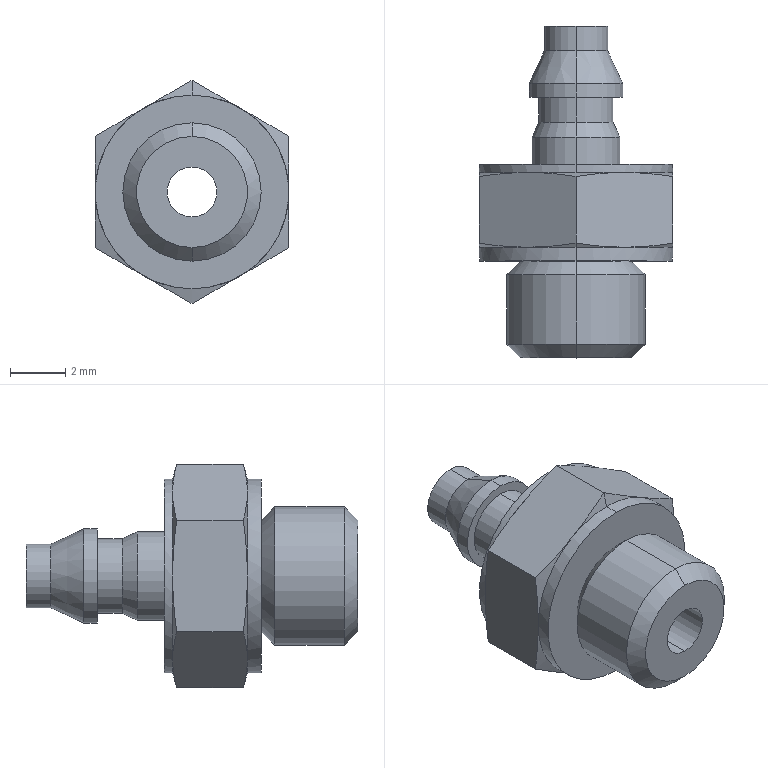Part | SolidWorks | features BaseBody 1 | 1 solid | 49 faces | box 7 x 12 x 8.083 mm | volume 212.301 mm3 | cone 22 | cylinder 16 | plane 11 | commonest cylinder face diameters 7 x4 1.8 x2 2.3 x2 2.7 x2 3.2 x2 3.4 x2
STEP:
#1=CARTESIAN_POINT('',(0.,-3.5,0.9));
#2=VERTEX_POINT('',#1);
#3=CARTESIAN_POINT('',(0.,-3.5,-0.9));
#4=VERTEX_POINT('',#3);
#5=CARTESIAN_POINT('',(0.,-3.5,0.));
#6=DIRECTION('',(0.,-1.,0.));
#7=DIRECTION('',(0.,0.,1.));
#8=AXIS2_PLACEMENT_3D('',#5,#6,#7);
#9=CIRCLE('',#8,0.9);
#10=EDGE_CURVE('',#2,#4,#9,.T.);
#11=ORIENTED_EDGE('',*,*,#10,.T.);
#12=CARTESIAN_POINT('',(0.,8.5,-0.9));
#13=VERTEX_POINT('',#12);
#14=CARTESIAN_POINT('',(0.,-3.5,-0.9));
#15=DIRECTION('',(0.,1.,0.));
#16=VECTOR('',#15,1000.);
#17=LINE('',#14,#16);
#18=EDGE_CURVE('',#4,#13,#17,.T.);
#19=ORIENTED_EDGE('',*,*,#18,.T.);
#20=CARTESIAN_POINT('',(0.,8.5,0.9));
#21=VERTEX_POINT('',#20);
#22=CARTESIAN_POINT('',(0.,8.5,0.));
#23=DIRECTION('',(0.,1.,0.));
#24=DIRECTION('',(0.,0.,1.));
#25=AXIS2_PLACEMENT_3D('',#22,#23,#24);
#26=CIRCLE('',#25,0.9);
#27=EDGE_CURVE('',#13,#21,#26,.T.);
#28=ORIENTED_EDGE('',*,*,#27,.T.);
#29=CARTESIAN_POINT('',(0.,-3.5,0.9));
#30=DIRECTION('',(0.,1.,0.));
#31=VECTOR('',#30,1000.);
#32=LINE('',#29,#31);
#33=EDGE_CURVE('',#2,#21,#32,.T.);
#34=ORIENTED_EDGE('',*,*,#33,.F.);
#35=EDGE_LOOP('',(#11,#19,#28,#34));
#36=FACE_OUTER_BOUND('',#35,.T.);
#37=CARTESIAN_POINT('',(0.,-3.5,0.));
#38=DIRECTION('',(0.,1.,0.));
#39=DIRECTION('',(0.,0.,1.));
#40=AXIS2_PLACEMENT_3D('',#37,#38,#39);
#41=CYLINDRICAL_SURFACE('',#40,0.9);
#42=ADVANCED_FACE('',(#36),#41,.F.);
#43=CARTESIAN_POINT('',(0.,7.6,1.15));
#44=VERTEX_POINT('',#43);
#45=CARTESIAN_POINT('',(0.,7.6,-1.15));
#46=VERTEX_POINT('',#45);
#47=CARTESIAN_POINT('',(0.,7.6,0.));
#48=DIRECTION('',(0.,1.,0.));
#49=DIRECTION('',(1.,0.,0.));
#50=AXIS2_PLACEMENT_3D('',#47,#48,#49);
#51=CIRCLE('',#50,1.15);
#52=EDGE_CURVE('',#44,#46,#51,.T.);
#53=ORIENTED_EDGE('',*,*,#52,.T.);
#54=CARTESIAN_POINT('',(0.,8.5,-1.15));
#55=VERTEX_POINT('',#54);
#56=CARTESIAN_POINT('',(0.,8.5,-1.15));
#57=DIRECTION('',(0.,1.,0.));
#58=VECTOR('',#57,1000.);
#59=LINE('',#56,#58);
#60=EDGE_CURVE('',#46,#55,#59,.T.);
#61=ORIENTED_EDGE('',*,*,#60,.T.);
#62=CARTESIAN_POINT('',(0.,8.5,1.15));
#63=VERTEX_POINT('',#62);
#64=CARTESIAN_POINT('',(0.,8.5,0.));
#65=DIRECTION('',(0.,1.,0.));
#66=DIRECTION('',(0.,0.,1.));
#67=AXIS2_PLACEMENT_3D('',#64,#65,#66);
#68=CIRCLE('',#67,1.15);
#69=EDGE_CURVE('',#63,#55,#68,.T.);
#70=ORIENTED_EDGE('',*,*,#69,.F.);
#71=CARTESIAN_POINT('',(0.,8.5,1.15));
#72=DIRECTION('',(0.,1.,0.));
#73=VECTOR('',#72,1000.);
#74=LINE('',#71,#73);
#75=EDGE_CURVE('',#44,#63,#74,.T.);
#76=ORIENTED_EDGE('',*,*,#75,.F.);
#77=EDGE_LOOP('',(#53,#61,#70,#76));
#78=FACE_OUTER_BOUND('',#77,.T.);
#79=CARTESIAN_POINT('',(0.,8.5,0.));
#80=DIRECTION('',(0.,1.,0.));
#81=DIRECTION('',(0.,0.,1.));
#82=AXIS2_PLACEMENT_3D('',#79,#80,#81);
#83=CYLINDRICAL_SURFACE('',#82,1.15);
#84=ADVANCED_FACE('',(#78),#83,.T.);
#85=CARTESIAN_POINT('',(0.,-3.5,-2.01));
#86=VERTEX_POINT('',#85);
#87=CARTESIAN_POINT('',(0.,-3.5,2.01));
#88=VERTEX_POINT('',#87);
#89=CARTESIAN_POINT('',(0.,-3.5,0.));
#90=DIRECTION('',(0.,-1.,0.));
#91=DIRECTION('',(0.,0.,1.));
#92=AXIS2_PLACEMENT_3D('',#89,#90,#91);
#93=CIRCLE('',#92,2.01);
#94=EDGE_CURVE('',#86,#88,#93,.T.);
#95=ORIENTED_EDGE('',*,*,#94,.F.);
#96=CARTESIAN_POINT('',(0.,-3.009,-2.5));
#97=VERTEX_POINT('',#96);
#98=CARTESIAN_POINT('',(0.,-3.5,-2.01));
#99=DIRECTION('',(0.,0.7071,-0.7071));
#100=VECTOR('',#99,1000.);
#101=LINE('',#98,#100);
#102=EDGE_CURVE('',#86,#97,#101,.T.);
#103=ORIENTED_EDGE('',*,*,#102,.T.);
#104=CARTESIAN_POINT('',(0.,-3.009,2.5));
#105=VERTEX_POINT('',#104);
#106=CARTESIAN_POINT('',(0.,-3.009,0.));
#107=DIRECTION('',(0.,-1.,0.));
#108=DIRECTION('',(1.,0.,0.));
#109=AXIS2_PLACEMENT_3D('',#106,#107,#108);
#110=CIRCLE('',#109,2.5);
#111=EDGE_CURVE('',#97,#105,#110,.T.);
#112=ORIENTED_EDGE('',*,*,#111,.T.);
#113=CARTESIAN_POINT('',(0.,-3.5,2.01));
#114=DIRECTION('',(0.,0.7071,0.7071));
#115=VECTOR('',#114,1000.);
#116=LINE('',#113,#115);
#117=EDGE_CURVE('',#88,#105,#116,.T.);
#118=ORIENTED_EDGE('',*,*,#117,.F.);
#119=EDGE_LOOP('',(#95,#103,#112,#118));
#120=FACE_OUTER_BOUND('',#119,.T.);
#121=CARTESIAN_POINT('',(0.,-3.5,0.));
#122=DIRECTION('',(0.,1.,0.));
#123=DIRECTION('',(0.,0.,1.));
#124=AXIS2_PLACEMENT_3D('',#121,#122,#123);
#125=CONICAL_SURFACE('',#124,2.01,0.7854);
#126=ADVANCED_FACE('',(#120),#125,.T.);
#127=ORIENTED_EDGE('',*,*,#52,.F.);
#128=CARTESIAN_POINT('',(0.,6.421,1.7));
#129=VERTEX_POINT('',#128);
#130=CARTESIAN_POINT('',(0.,7.6,1.15));
#131=DIRECTION('',(0.,-0.9063,0.4226));
#132=VECTOR('',#131,1000.);
#133=LINE('',#130,#132);
#134=EDGE_CURVE('',#44,#129,#133,.T.);
#135=ORIENTED_EDGE('',*,*,#134,.T.);
#136=CARTESIAN_POINT('',(0.,6.421,-1.7));
#137=VERTEX_POINT('',#136);
#138=CARTESIAN_POINT('',(0.,6.421,0.));
#139=DIRECTION('',(0.,1.,0.));
#140=DIRECTION('',(1.,0.,0.));
#141=AXIS2_PLACEMENT_3D('',#138,#139,#140);
#142=CIRCLE('',#141,1.7);
#143=EDGE_CURVE('',#129,#137,#142,.T.);
#144=ORIENTED_EDGE('',*,*,#143,.T.);
#145=CARTESIAN_POINT('',(0.,7.6,-1.15));
#146=DIRECTION('',(0.,-0.9063,-0.4226));
#147=VECTOR('',#146,1000.);
#148=LINE('',#145,#147);
#149=EDGE_CURVE('',#46,#137,#148,.T.);
#150=ORIENTED_EDGE('',*,*,#149,.F.);
#151=EDGE_LOOP('',(#127,#135,#144,#150));
#152=FACE_OUTER_BOUND('',#151,.T.);
#153=CARTESIAN_POINT('',(0.,7.6,0.));
#154=DIRECTION('',(0.,-1.,0.));
#155=DIRECTION('',(0.,0.,-1.));
#156=AXIS2_PLACEMENT_3D('',#153,#154,#155);
#157=CONICAL_SURFACE('',#156,1.15,0.4363);
#158=ADVANCED_FACE('',(#152),#157,.T.);
#159=ORIENTED_EDGE('',*,*,#111,.F.);
#160=CARTESIAN_POINT('',(0.,-0.4905,-2.5));
#161=VERTEX_POINT('',#160);
#162=CARTESIAN_POINT('',(0.,-0.4905,-2.5));
#163=DIRECTION('',(0.,1.,0.));
#164=VECTOR('',#163,1000.);
#165=LINE('',#162,#164);
#166=EDGE_CURVE('',#97,#161,#165,.T.);
#167=ORIENTED_EDGE('',*,*,#166,.T.);
#168=CARTESIAN_POINT('',(0.,-0.4905,2.5));
#169=VERTEX_POINT('',#168);
#170=CARTESIAN_POINT('',(0.,-0.4905,0.));
#171=DIRECTION('',(0.,-1.,0.));
#172=DIRECTION('',(1.,0.,0.));
#173=AXIS2_PLACEMENT_3D('',#170,#171,#172);
#174=CIRCLE('',#173,2.5);
#175=EDGE_CURVE('',#161,#169,#174,.T.);
#176=ORIENTED_EDGE('',*,*,#175,.T.);
#177=CARTESIAN_POINT('',(0.,-0.4905,2.5));
#178=DIRECTION('',(0.,1.,0.));
#179=VECTOR('',#178,1000.);
#180=LINE('',#177,#179);
#181=EDGE_CURVE('',#105,#169,#180,.T.);
#182=ORIENTED_EDGE('',*,*,#181,.F.);
#183=EDGE_LOOP('',(#159,#167,#176,#182));
#184=FACE_OUTER_BOUND('',#183,.T.);
#185=CARTESIAN_POINT('',(0.,-0.4905,0.));
#186=DIRECTION('',(0.,1.,0.));
#187=DIRECTION('',(0.,0.,1.));
#188=AXIS2_PLACEMENT_3D('',#185,#186,#187);
#189=CYLINDRICAL_SURFACE('',#188,2.5);
#190=ADVANCED_FACE('',(#184),#189,.T.);
#191=CARTESIAN_POINT('',(0.,5.921,1.7));
#192=VERTEX_POINT('',#191);
#193=CARTESIAN_POINT('',(0.,5.921,-1.7));
#194=VERTEX_POINT('',#193);
#195=CARTESIAN_POINT('',(0.,5.921,0.));
#196=DIRECTION('',(0.,1.,0.));
#197=DIRECTION('',(0.,0.,1.));
#198=AXIS2_PLACEMENT_3D('',#195,#196,#197);
#199=CIRCLE('',#198,1.7);
#200=EDGE_CURVE('',#192,#194,#199,.T.);
#201=ORIENTED_EDGE('',*,*,#200,.T.);
#202=CARTESIAN_POINT('',(0.,6.421,-1.7));
#203=DIRECTION('',(0.,1.,0.));
#204=VECTOR('',#203,1000.);
#205=LINE('',#202,#204);
#206=EDGE_CURVE('',#194,#137,#205,.T.);
#207=ORIENTED_EDGE('',*,*,#206,.T.);
#208=ORIENTED_EDGE('',*,*,#143,.F.);
#209=CARTESIAN_POINT('',(0.,6.421,1.7));
#210=DIRECTION('',(0.,1.,0.));
#211=VECTOR('',#210,1000.);
#212=LINE('',#209,#211);
#213=EDGE_CURVE('',#192,#129,#212,.T.);
#214=ORIENTED_EDGE('',*,*,#213,.F.);
#215=EDGE_LOOP('',(#201,#207,#208,#214));
#216=FACE_OUTER_BOUND('',#215,.T.);
#217=CARTESIAN_POINT('',(0.,6.421,0.));
#218=DIRECTION('',(0.,1.,0.));
#219=DIRECTION('',(0.,0.,1.));
#220=AXIS2_PLACEMENT_3D('',#217,#218,#219);
#221=CYLINDRICAL_SURFACE('',#220,1.7);
#222=ADVANCED_FACE('',(#216),#221,.T.);
#223=CARTESIAN_POINT('',(0.,0.,-2.01));
#224=VERTEX_POINT('',#223);
#225=CARTESIAN_POINT('',(0.,0.,2.01));
#226=VERTEX_POINT('',#225);
#227=CARTESIAN_POINT('',(0.,0.,0.));
#228=DIRECTION('',(0.,-1.,0.));
#229=DIRECTION('',(0.,0.,-1.));
#230=AXIS2_PLACEMENT_3D('',#227,#228,#229);
#231=CIRCLE('',#230,2.01);
#232=EDGE_CURVE('',#224,#226,#231,.T.);
#233=ORIENTED_EDGE('',*,*,#232,.T.);
#234=CARTESIAN_POINT('',(0.,0.,2.01));
#235=DIRECTION('',(0.,-0.7071,0.7071));
#236=VECTOR('',#235,1000.);
#237=LINE('',#234,#236);
#238=EDGE_CURVE('',#226,#169,#237,.T.);
#239=ORIENTED_EDGE('',*,*,#238,.T.);
#240=ORIENTED_EDGE('',*,*,#175,.F.);
#241=CARTESIAN_POINT('',(0.,0.,-2.01));
#242=DIRECTION('',(0.,-0.7071,-0.7071));
#243=VECTOR('',#242,1000.);
#244=LINE('',#241,#243);
#245=EDGE_CURVE('',#224,#161,#244,.T.);
#246=ORIENTED_EDGE('',*,*,#245,.F.);
#247=EDGE_LOOP('',(#233,#239,#240,#246));
#248=FACE_OUTER_BOUND('',#247,.T.);
#249=CARTESIAN_POINT('',(0.,0.,0.));
#250=DIRECTION('',(0.,-1.,0.));
#251=DIRECTION('',(0.,0.,-1.));
#252=AXIS2_PLACEMENT_3D('',#249,#250,#251);
#253=CONICAL_SURFACE('',#252,2.01,0.7854);
#254=ADVANCED_FACE('',(#248),#253,.T.);
#255=CARTESIAN_POINT('',(0.,5.021,1.35));
#256=VERTEX_POINT('',#255);
#257=CARTESIAN_POINT('',(0.,5.021,-1.35));
#258=VERTEX_POINT('',#257);
#259=CARTESIAN_POINT('',(0.,5.021,0.));
#260=DIRECTION('',(0.,1.,0.));
#261=DIRECTION('',(1.,0.,0.));
#262=AXIS2_PLACEMENT_3D('',#259,#260,#261);
#263=CIRCLE('',#262,1.35);
#264=EDGE_CURVE('',#256,#258,#263,.T.);
#265=ORIENTED_EDGE('',*,*,#264,.T.);
#266=CARTESIAN_POINT('',(0.,5.921,-1.35));
#267=VERTEX_POINT('',#266);
#268=CARTESIAN_POINT('',(0.,5.921,-1.35));
#269=DIRECTION('',(0.,1.,0.));
#270=VECTOR('',#269,1000.);
#271=LINE('',#268,#270);
#272=EDGE_CURVE('',#258,#267,#271,.T.);
#273=ORIENTED_EDGE('',*,*,#272,.T.);
#274=CARTESIAN_POINT('',(0.,5.921,1.35));
#275=VERTEX_POINT('',#274);
#276=CARTESIAN_POINT('',(0.,5.921,0.));
#277=DIRECTION('',(0.,1.,0.));
#278=DIRECTION('',(0.,0.,1.));
#279=AXIS2_PLACEMENT_3D('',#276,#277,#278);
#280=CIRCLE('',#279,1.35);
#281=EDGE_CURVE('',#275,#267,#280,.T.);
#282=ORIENTED_EDGE('',*,*,#281,.F.);
#283=CARTESIAN_POINT('',(0.,5.921,1.35));
#284=DIRECTION('',(0.,1.,0.));
#285=VECTOR('',#284,1000.);
#286=LINE('',#283,#285);
#287=EDGE_CURVE('',#256,#275,#286,.T.);
#288=ORIENTED_EDGE('',*,*,#287,.F.);
#289=EDGE_LOOP('',(#265,#273,#282,#288));
#290=FACE_OUTER_BOUND('',#289,.T.);
#291=CARTESIAN_POINT('',(0.,5.921,0.));
#292=DIRECTION('',(0.,1.,0.));
#293=DIRECTION('',(0.,0.,1.));
#294=AXIS2_PLACEMENT_3D('',#291,#292,#293);
#295=CYLINDRICAL_SURFACE('',#294,1.35);
#296=ADVANCED_FACE('',(#290),#295,.T.);
#297=CARTESIAN_POINT('',(0.,0.,-3.5));
#298=VERTEX_POINT('',#297);
#299=CARTESIAN_POINT('',(0.,0.,3.5));
#300=VERTEX_POINT('',#299);
#301=CARTESIAN_POINT('',(0.,0.,0.));
#302=DIRECTION('',(0.,-1.,0.));
#303=DIRECTION('',(0.,0.,1.));
#304=AXIS2_PLACEMENT_3D('',#301,#302,#303);
#305=CIRCLE('',#304,3.5);
#306=EDGE_CURVE('',#298,#300,#305,.T.);
#307=ORIENTED_EDGE('',*,*,#306,.F.);
#308=CARTESIAN_POINT('',(0.,0.5,-3.5));
#309=VERTEX_POINT('',#308);
#310=CARTESIAN_POINT('',(0.,0.5,-3.5));
#311=DIRECTION('',(0.,1.,0.));
#312=VECTOR('',#311,1000.);
#313=LINE('',#310,#312);
#314=EDGE_CURVE('',#298,#309,#313,.T.);
#315=ORIENTED_EDGE('',*,*,#314,.T.);
#316=CARTESIAN_POINT('',(1.75,0.5,-3.031));
#317=VERTEX_POINT('',#316);
#318=CARTESIAN_POINT('',(0.,0.5,0.));
#319=DIRECTION('',(0.,-1.,0.));
#320=DIRECTION('',(1.,0.,0.));
#321=AXIS2_PLACEMENT_3D('',#318,#319,#320);
#322=CIRCLE('',#321,3.5);
#323=EDGE_CURVE('',#309,#317,#322,.T.);
#324=ORIENTED_EDGE('',*,*,#323,.T.);
#325=CARTESIAN_POINT('',(3.5,0.5,0.));
#326=VERTEX_POINT('',#325);
#327=CARTESIAN_POINT('',(0.,0.5,0.));
#328=DIRECTION('',(0.,-1.,0.));
#329=DIRECTION('',(1.,0.,0.));
#330=AXIS2_PLACEMENT_3D('',#327,#328,#329);
#331=CIRCLE('',#330,3.5);
#332=EDGE_CURVE('',#317,#326,#331,.T.);
#333=ORIENTED_EDGE('',*,*,#332,.T.);
#334=CARTESIAN_POINT('',(1.75,0.5,3.031));
#335=VERTEX_POINT('',#334);
#336=CARTESIAN_POINT('',(0.,0.5,0.));
#337=DIRECTION('',(0.,-1.,0.));
#338=DIRECTION('',(1.,0.,0.));
#339=AXIS2_PLACEMENT_3D('',#336,#337,#338);
#340=CIRCLE('',#339,3.5);
#341=EDGE_CURVE('',#326,#335,#340,.T.);
#342=ORIENTED_EDGE('',*,*,#341,.T.);
#343=CARTESIAN_POINT('',(0.,0.5,3.5));
#344=VERTEX_POINT('',#343);
#345=CARTESIAN_POINT('',(0.,0.5,0.));
#346=DIRECTION('',(0.,-1.,0.));
#347=DIRECTION('',(1.,0.,0.));
#348=AXIS2_PLACEMENT_3D('',#345,#346,#347);
#349=CIRCLE('',#348,3.5);
#350=EDGE_CURVE('',#335,#344,#349,.T.);
#351=ORIENTED_EDGE('',*,*,#350,.T.);
#352=CARTESIAN_POINT('',(0.,0.5,3.5));
#353=DIRECTION('',(0.,1.,0.));
#354=VECTOR('',#353,1000.);
#355=LINE('',#352,#354);
#356=EDGE_CURVE('',#300,#344,#355,.T.);
#357=ORIENTED_EDGE('',*,*,#356,.F.);
#358=EDGE_LOOP('',(#307,#315,#324,#333,#342,#351,#357));
#359=FACE_OUTER_BOUND('',#358,.T.);
#360=CARTESIAN_POINT('',(0.,0.5,0.));
#361=DIRECTION('',(0.,1.,0.));
#362=DIRECTION('',(0.,0.,1.));
#363=AXIS2_PLACEMENT_3D('',#360,#361,#362);
#364=CYLINDRICAL_SURFACE('',#363,3.5);
#365=ADVANCED_FACE('',(#359),#364,.T.);
#366=ORIENTED_EDGE('',*,*,#264,.F.);
#367=CARTESIAN_POINT('',(0.,4.484,1.6));
#368=VERTEX_POINT('',#367);
#369=CARTESIAN_POINT('',(0.,5.021,1.35));
#370=DIRECTION('',(0.,-0.9063,0.4226));
#371=VECTOR('',#370,1000.);
#372=LINE('',#369,#371);
#373=EDGE_CURVE('',#256,#368,#372,.T.);
#374=ORIENTED_EDGE('',*,*,#373,.T.);
#375=CARTESIAN_POINT('',(0.,4.484,-1.6));
#376=VERTEX_POINT('',#375);
#377=CARTESIAN_POINT('',(0.,4.484,0.));
#378=DIRECTION('',(0.,1.,0.));
#379=DIRECTION('',(1.,0.,0.));
#380=AXIS2_PLACEMENT_3D('',#377,#378,#379);
#381=CIRCLE('',#380,1.6);
#382=EDGE_CURVE('',#368,#376,#381,.T.);
#383=ORIENTED_EDGE('',*,*,#382,.T.);
#384=CARTESIAN_POINT('',(0.,5.021,-1.35));
#385=DIRECTION('',(0.,-0.9063,-0.4226));
#386=VECTOR('',#385,1000.);
#387=LINE('',#384,#386);
#388=EDGE_CURVE('',#258,#376,#387,.T.);
#389=ORIENTED_EDGE('',*,*,#388,.F.);
#390=EDGE_LOOP('',(#366,#374,#383,#389));
#391=FACE_OUTER_BOUND('',#390,.T.);
#392=CARTESIAN_POINT('',(0.,5.021,0.));
#393=DIRECTION('',(0.,-1.,0.));
#394=DIRECTION('',(0.,0.,-1.));
#395=AXIS2_PLACEMENT_3D('',#392,#393,#394);
#396=CONICAL_SURFACE('',#395,1.35,0.4363);
#397=ADVANCED_FACE('',(#391),#396,.T.);
#398=CARTESIAN_POINT('',(-1.75,0.5,3.031));
#399=VERTEX_POINT('',#398);
#400=CARTESIAN_POINT('',(0.,0.5,0.));
#401=DIRECTION('',(0.,-1.,0.));
#402=DIRECTION('',(1.,0.,0.));
#403=AXIS2_PLACEMENT_3D('',#400,#401,#402);
#404=CIRCLE('',#403,3.5);
#405=EDGE_CURVE('',#344,#399,#404,.T.);
#406=ORIENTED_EDGE('',*,*,#405,.F.);
#407=CARTESIAN_POINT('',(0.,0.6451,4.041));
#408=VERTEX_POINT('',#407);
#409=CARTESIAN_POINT('',(0.,0.5,3.5));
#410=DIRECTION('',(0.,0.2588,0.9659));
#411=VECTOR('',#410,1000.);
#412=LINE('',#409,#411);
#413=EDGE_CURVE('',#344,#408,#412,.T.);
#414=ORIENTED_EDGE('',*,*,#413,.T.);
#415=CARTESIAN_POINT('',(0.,0.6451,4.041));
#416=CARTESIAN_POINT('',(-0.5808,0.5552,3.706));
#417=CARTESIAN_POINT('',(-1.164,0.5,3.37));
#418=CARTESIAN_POINT('',(-1.75,0.5,3.031));
#419=B_SPLINE_CURVE_WITH_KNOTS('',3,(#415,#416,#417,#418),.UNSPECIFIED.,.F.,.F.,(4,4),(0.,0.002026),.UNSPECIFIED.);
#420=EDGE_CURVE('',#408,#399,#419,.T.);
#421=ORIENTED_EDGE('',*,*,#420,.T.);
#422=EDGE_LOOP('',(#406,#414,#421));
#423=FACE_OUTER_BOUND('',#422,.T.);
#424=CARTESIAN_POINT('',(0.,0.5,0.));
#425=DIRECTION('',(0.,1.,0.));
#426=DIRECTION('',(0.,0.,1.));
#427=AXIS2_PLACEMENT_3D('',#424,#425,#426);
#428=CONICAL_SURFACE('',#427,3.5,1.309);
#429=ADVANCED_FACE('',(#423),#428,.T.);
#430=CARTESIAN_POINT('',(0.,3.5,1.6));
#431=VERTEX_POINT('',#430);
#432=CARTESIAN_POINT('',(0.,3.5,-1.6));
#433=VERTEX_POINT('',#432);
#434=CARTESIAN_POINT('',(0.,3.5,0.));
#435=DIRECTION('',(0.,1.,0.));
#436=DIRECTION('',(0.,0.,1.));
#437=AXIS2_PLACEMENT_3D('',#434,#435,#436);
#438=CIRCLE('',#437,1.6);
#439=EDGE_CURVE('',#431,#433,#438,.T.);
#440=ORIENTED_EDGE('',*,*,#439,.T.);
#441=CARTESIAN_POINT('',(0.,4.484,-1.6));
#442=DIRECTION('',(0.,1.,0.));
#443=VECTOR('',#442,1000.);
#444=LINE('',#441,#443);
#445=EDGE_CURVE('',#433,#376,#444,.T.);
#446=ORIENTED_EDGE('',*,*,#445,.T.);
#447=ORIENTED_EDGE('',*,*,#382,.F.);
#448=CARTESIAN_POINT('',(0.,4.484,1.6));
#449=DIRECTION('',(0.,1.,0.));
#450=VECTOR('',#449,1000.);
#451=LINE('',#448,#450);
#452=EDGE_CURVE('',#431,#368,#451,.T.);
#453=ORIENTED_EDGE('',*,*,#452,.F.);
#454=EDGE_LOOP('',(#440,#446,#447,#453));
#455=FACE_OUTER_BOUND('',#454,.T.);
#456=CARTESIAN_POINT('',(0.,4.484,0.));
#457=DIRECTION('',(0.,1.,0.));
#458=DIRECTION('',(0.,0.,1.));
#459=AXIS2_PLACEMENT_3D('',#456,#457,#458);
#460=CYLINDRICAL_SURFACE('',#459,1.6);
#461=ADVANCED_FACE('',(#455),#460,.T.);
#462=CARTESIAN_POINT('',(-1.75,3.2,-3.031));
#463=VERTEX_POINT('',#462);
#464=CARTESIAN_POINT('',(0.,3.2,-3.5));
#465=VERTEX_POINT('',#464);
#466=CARTESIAN_POINT('',(0.,3.2,0.));
#467=DIRECTION('',(0.,-1.,0.));
#468=DIRECTION('',(1.,0.,0.));
#469=AXIS2_PLACEMENT_3D('',#466,#467,#468);
#470=CIRCLE('',#469,3.5);
#471=EDGE_CURVE('',#463,#465,#470,.T.);
#472=ORIENTED_EDGE('',*,*,#471,.T.);
#473=CARTESIAN_POINT('',(0.,3.055,-4.041));
#474=VERTEX_POINT('',#473);
#475=CARTESIAN_POINT('',(0.,3.2,-3.5));
#476=DIRECTION('',(0.,-0.2588,-0.9659));
#477=VECTOR('',#476,1000.);
#478=LINE('',#475,#477);
#479=EDGE_CURVE('',#465,#474,#478,.T.);
#480=ORIENTED_EDGE('',*,*,#479,.T.);
#481=CARTESIAN_POINT('',(-1.75,3.2,-3.031));
#482=CARTESIAN_POINT('',(-1.164,3.2,-3.37));
#483=CARTESIAN_POINT('',(-0.5808,3.145,-3.706));
#484=CARTESIAN_POINT('',(0.,3.055,-4.041));
#485=B_SPLINE_CURVE_WITH_KNOTS('',3,(#481,#482,#483,#484),.UNSPECIFIED.,.F.,.F.,(4,4),(0.,0.002026),.UNSPECIFIED.);
#486=EDGE_CURVE('',#463,#474,#485,.T.);
#487=ORIENTED_EDGE('',*,*,#486,.F.);
#488=EDGE_LOOP('',(#472,#480,#487));
#489=FACE_OUTER_BOUND('',#488,.T.);
#490=CARTESIAN_POINT('',(0.,3.2,0.));
#491=DIRECTION('',(0.,-1.,0.));
#492=DIRECTION('',(0.,0.,-1.));
#493=AXIS2_PLACEMENT_3D('',#490,#491,#492);
#494=CONICAL_SURFACE('',#493,3.5,1.309);
#495=ADVANCED_FACE('',(#489),#494,.T.);
#496=CARTESIAN_POINT('',(1.75,3.2,-3.031));
#497=VERTEX_POINT('',#496);
#498=CARTESIAN_POINT('',(0.,3.2,0.));
#499=DIRECTION('',(0.,-1.,0.));
#500=DIRECTION('',(1.,0.,0.));
#501=AXIS2_PLACEMENT_3D('',#498,#499,#500);
#502=CIRCLE('',#501,3.5);
#503=EDGE_CURVE('',#465,#497,#502,.T.);
#504=ORIENTED_EDGE('',*,*,#503,.F.);
#505=CARTESIAN_POINT('',(0.,3.5,-3.5));
#506=VERTEX_POINT('',#505);
#507=CARTESIAN_POINT('',(0.,3.5,-3.5));
#508=DIRECTION('',(0.,1.,0.));
#509=VECTOR('',#508,1000.);
#510=LINE('',#507,#509);
#511=EDGE_CURVE('',#465,#506,#510,.T.);
#512=ORIENTED_EDGE('',*,*,#511,.T.);
#513=CARTESIAN_POINT('',(0.,3.5,3.5));
#514=VERTEX_POINT('',#513);
#515=CARTESIAN_POINT('',(0.,3.5,0.));
#516=DIRECTION('',(0.,1.,0.));
#517=DIRECTION('',(0.,0.,1.));
#518=AXIS2_PLACEMENT_3D('',#515,#516,#517);
#519=CIRCLE('',#518,3.5);
#520=EDGE_CURVE('',#514,#506,#519,.T.);
#521=ORIENTED_EDGE('',*,*,#520,.F.);
#522=CARTESIAN_POINT('',(0.,3.2,3.5));
#523=VERTEX_POINT('',#522);
#524=CARTESIAN_POINT('',(0.,3.5,3.5));
#525=DIRECTION('',(0.,1.,0.));
#526=VECTOR('',#525,1000.);
#527=LINE('',#524,#526);
#528=EDGE_CURVE('',#523,#514,#527,.T.);
#529=ORIENTED_EDGE('',*,*,#528,.F.);
#530=CARTESIAN_POINT('',(1.75,3.2,3.031));
#531=VERTEX_POINT('',#530);
#532=CARTESIAN_POINT('',(0.,3.2,0.));
#533=DIRECTION('',(0.,-1.,0.));
#534=DIRECTION('',(1.,0.,0.));
#535=AXIS2_PLACEMENT_3D('',#532,#533,#534);
#536=CIRCLE('',#535,3.5);
#537=EDGE_CURVE('',#531,#523,#536,.T.);
#538=ORIENTED_EDGE('',*,*,#537,.F.);
#539=CARTESIAN_POINT('',(3.5,3.2,0.));
#540=VERTEX_POINT('',#539);
#541=CARTESIAN_POINT('',(0.,3.2,0.));
#542=DIRECTION('',(0.,-1.,0.));
#543=DIRECTION('',(1.,0.,0.));
#544=AXIS2_PLACEMENT_3D('',#541,#542,#543);
#545=CIRCLE('',#544,3.5);
#546=EDGE_CURVE('',#540,#531,#545,.T.);
#547=ORIENTED_EDGE('',*,*,#546,.F.);
#548=CARTESIAN_POINT('',(0.,3.2,0.));
#549=DIRECTION('',(0.,-1.,0.));
#550=DIRECTION('',(1.,0.,0.));
#551=AXIS2_PLACEMENT_3D('',#548,#549,#550);
#552=CIRCLE('',#551,3.5);
#553=EDGE_CURVE('',#497,#540,#552,.T.);
#554=ORIENTED_EDGE('',*,*,#553,.F.);
#555=EDGE_LOOP('',(#504,#512,#521,#529,#538,#547,#554));
#556=FACE_OUTER_BOUND('',#555,.T.);
#557=CARTESIAN_POINT('',(0.,3.5,0.));
#558=DIRECTION('',(0.,1.,0.));
#559=DIRECTION('',(0.,0.,1.));
#560=AXIS2_PLACEMENT_3D('',#557,#558,#559);
#561=CYLINDRICAL_SURFACE('',#560,3.5);
#562=ADVANCED_FACE('',(#556),#561,.T.);
#563=ORIENTED_EDGE('',*,*,#18,.F.);
#564=CARTESIAN_POINT('',(0.,-3.5,0.));
#565=DIRECTION('',(0.,-1.,0.));
#566=DIRECTION('',(0.,0.,1.));
#567=AXIS2_PLACEMENT_3D('',#564,#565,#566);
#568=CIRCLE('',#567,0.9);
#569=EDGE_CURVE('',#4,#2,#568,.T.);
#570=ORIENTED_EDGE('',*,*,#569,.T.);
#571=ORIENTED_EDGE('',*,*,#33,.T.);
#572=CARTESIAN_POINT('',(0.,8.5,0.));
#573=DIRECTION('',(0.,1.,0.));
#574=DIRECTION('',(0.,0.,1.));
#575=AXIS2_PLACEMENT_3D('',#572,#573,#574);
#576=CIRCLE('',#575,0.9);
#577=EDGE_CURVE('',#21,#13,#576,.T.);
#578=ORIENTED_EDGE('',*,*,#577,.T.);
#579=EDGE_LOOP('',(#563,#570,#571,#578));
#580=FACE_OUTER_BOUND('',#579,.T.);
#581=CARTESIAN_POINT('',(0.,-3.5,0.));
#582=DIRECTION('',(0.,1.,0.));
#583=DIRECTION('',(0.,0.,1.));
#584=AXIS2_PLACEMENT_3D('',#581,#582,#583);
#585=CYLINDRICAL_SURFACE('',#584,0.9);
#586=ADVANCED_FACE('',(#580),#585,.F.);
#587=ORIENTED_EDGE('',*,*,#577,.F.);
#588=ORIENTED_EDGE('',*,*,#27,.F.);
#589=EDGE_LOOP('',(#587,#588));
#590=FACE_BOUND('',#589,.T.);
#591=ORIENTED_EDGE('',*,*,#69,.T.);
#592=CARTESIAN_POINT('',(0.,8.5,0.));
#593=DIRECTION('',(0.,1.,0.));
#594=DIRECTION('',(0.,0.,1.));
#595=AXIS2_PLACEMENT_3D('',#592,#593,#594);
#596=CIRCLE('',#595,1.15);
#597=EDGE_CURVE('',#55,#63,#596,.T.);
#598=ORIENTED_EDGE('',*,*,#597,.T.);
#599=EDGE_LOOP('',(#591,#598));
#600=FACE_OUTER_BOUND('',#599,.T.);
#601=CARTESIAN_POINT('',(-1.15,8.5,1.164));
#602=DIRECTION('',(0.,1.,0.));
#603=DIRECTION('',(1.,0.,0.));
#604=AXIS2_PLACEMENT_3D('',#601,#602,#603);
#605=PLANE('',#604);
#606=ADVANCED_FACE('',(#590,#600),#605,.T.);
#607=ORIENTED_EDGE('',*,*,#10,.F.);
#608=ORIENTED_EDGE('',*,*,#569,.F.);
#609=EDGE_LOOP('',(#607,#608));
#610=FACE_BOUND('',#609,.T.);
#611=CARTESIAN_POINT('',(0.,-3.5,0.));
#612=DIRECTION('',(0.,-1.,0.));
#613=DIRECTION('',(0.,0.,1.));
#614=AXIS2_PLACEMENT_3D('',#611,#612,#613);
#615=CIRCLE('',#614,2.01);
#616=EDGE_CURVE('',#88,#86,#615,.T.);
#617=ORIENTED_EDGE('',*,*,#616,.T.);
#618=ORIENTED_EDGE('',*,*,#94,.T.);
#619=EDGE_LOOP('',(#617,#618));
#620=FACE_OUTER_BOUND('',#619,.T.);
#621=CARTESIAN_POINT('',(2.01,-3.5,2.034));
#622=DIRECTION('',(0.,-1.,0.));
#623=DIRECTION('',(-1.,0.,0.));
#624=AXIS2_PLACEMENT_3D('',#621,#622,#623);
#625=PLANE('',#624);
#626=ADVANCED_FACE('',(#610,#620),#625,.T.);
#627=ORIENTED_EDGE('',*,*,#60,.F.);
#628=CARTESIAN_POINT('',(0.,7.6,0.));
#629=DIRECTION('',(0.,1.,0.));
#630=DIRECTION('',(1.,0.,0.));
#631=AXIS2_PLACEMENT_3D('',#628,#629,#630);
#632=CIRCLE('',#631,1.15);
#633=EDGE_CURVE('',#46,#44,#632,.T.);
#634=ORIENTED_EDGE('',*,*,#633,.T.);
#635=ORIENTED_EDGE('',*,*,#75,.T.);
#636=ORIENTED_EDGE('',*,*,#597,.F.);
#637=EDGE_LOOP('',(#627,#634,#635,#636));
#638=FACE_OUTER_BOUND('',#637,.T.);
#639=CARTESIAN_POINT('',(0.,8.5,0.));
#640=DIRECTION('',(0.,1.,0.));
#641=DIRECTION('',(0.,0.,1.));
#642=AXIS2_PLACEMENT_3D('',#639,#640,#641);
#643=CYLINDRICAL_SURFACE('',#642,1.15);
#644=ADVANCED_FACE('',(#638),#643,.T.);
#645=ORIENTED_EDGE('',*,*,#102,.F.);
#646=ORIENTED_EDGE('',*,*,#616,.F.);
#647=ORIENTED_EDGE('',*,*,#117,.T.);
#648=CARTESIAN_POINT('',(0.,-3.009,0.));
#649=DIRECTION('',(0.,-1.,0.));
#650=DIRECTION('',(1.,0.,0.));
#651=AXIS2_PLACEMENT_3D('',#648,#649,#650);
#652=CIRCLE('',#651,2.5);
#653=EDGE_CURVE('',#105,#97,#652,.T.);
#654=ORIENTED_EDGE('',*,*,#653,.T.);
#655=EDGE_LOOP('',(#645,#646,#647,#654));
#656=FACE_OUTER_BOUND('',#655,.T.);
#657=CARTESIAN_POINT('',(0.,-3.5,0.));
#658=DIRECTION('',(0.,1.,0.));
#659=DIRECTION('',(0.,0.,1.));
#660=AXIS2_PLACEMENT_3D('',#657,#658,#659);
#661=CONICAL_SURFACE('',#660,2.01,0.7854);
#662=ADVANCED_FACE('',(#656),#661,.T.);
#663=ORIENTED_EDGE('',*,*,#134,.F.);
#664=ORIENTED_EDGE('',*,*,#633,.F.);
#665=ORIENTED_EDGE('',*,*,#149,.T.);
#666=CARTESIAN_POINT('',(0.,6.421,0.));
#667=DIRECTION('',(0.,1.,0.));
#668=DIRECTION('',(1.,0.,0.));
#669=AXIS2_PLACEMENT_3D('',#666,#667,#668);
#670=CIRCLE('',#669,1.7);
#671=EDGE_CURVE('',#137,#129,#670,.T.);
#672=ORIENTED_EDGE('',*,*,#671,.T.);
#673=EDGE_LOOP('',(#663,#664,#665,#672));
#674=FACE_OUTER_BOUND('',#673,.T.);
#675=CARTESIAN_POINT('',(0.,7.6,0.));
#676=DIRECTION('',(0.,-1.,0.));
#677=DIRECTION('',(0.,0.,-1.));
#678=AXIS2_PLACEMENT_3D('',#675,#676,#677);
#679=CONICAL_SURFACE('',#678,1.15,0.4363);
#680=ADVANCED_FACE('',(#674),#679,.T.);
#681=ORIENTED_EDGE('',*,*,#166,.F.);
#682=ORIENTED_EDGE('',*,*,#653,.F.);
#683=ORIENTED_EDGE('',*,*,#181,.T.);
#684=CARTESIAN_POINT('',(0.,-0.4905,0.));
#685=DIRECTION('',(0.,-1.,0.));
#686=DIRECTION('',(1.,0.,0.));
#687=AXIS2_PLACEMENT_3D('',#684,#685,#686);
#688=CIRCLE('',#687,2.5);
#689=EDGE_CURVE('',#169,#161,#688,.T.);
#690=ORIENTED_EDGE('',*,*,#689,.T.);
#691=EDGE_LOOP('',(#681,#682,#683,#690));
#692=FACE_OUTER_BOUND('',#691,.T.);
#693=CARTESIAN_POINT('',(0.,-0.4905,0.));
#694=DIRECTION('',(0.,1.,0.));
#695=DIRECTION('',(0.,0.,1.));
#696=AXIS2_PLACEMENT_3D('',#693,#694,#695);
#697=CYLINDRICAL_SURFACE('',#696,2.5);
#698=ADVANCED_FACE('',(#692),#697,.T.);
#699=ORIENTED_EDGE('',*,*,#206,.F.);
#700=CARTESIAN_POINT('',(0.,5.921,0.));
#701=DIRECTION('',(0.,1.,0.));
#702=DIRECTION('',(0.,0.,1.));
#703=AXIS2_PLACEMENT_3D('',#700,#701,#702);
#704=CIRCLE('',#703,1.7);
#705=EDGE_CURVE('',#194,#192,#704,.T.);
#706=ORIENTED_EDGE('',*,*,#705,.T.);
#707=ORIENTED_EDGE('',*,*,#213,.T.);
#708=ORIENTED_EDGE('',*,*,#671,.F.);
#709=EDGE_LOOP('',(#699,#706,#707,#708));
#710=FACE_OUTER_BOUND('',#709,.T.);
#711=CARTESIAN_POINT('',(0.,6.421,0.));
#712=DIRECTION('',(0.,1.,0.));
#713=DIRECTION('',(0.,0.,1.));
#714=AXIS2_PLACEMENT_3D('',#711,#712,#713);
#715=CYLINDRICAL_SURFACE('',#714,1.7);
#716=ADVANCED_FACE('',(#710),#715,.T.);
#717=ORIENTED_EDGE('',*,*,#238,.F.);
#718=CARTESIAN_POINT('',(0.,0.,0.));
#719=DIRECTION('',(0.,-1.,0.));
#720=DIRECTION('',(0.,0.,-1.));
#721=AXIS2_PLACEMENT_3D('',#718,#719,#720);
#722=CIRCLE('',#721,2.01);
#723=EDGE_CURVE('',#226,#224,#722,.T.);
#724=ORIENTED_EDGE('',*,*,#723,.T.);
#725=ORIENTED_EDGE('',*,*,#245,.T.);
#726=ORIENTED_EDGE('',*,*,#689,.F.);
#727=EDGE_LOOP('',(#717,#724,#725,#726));
#728=FACE_OUTER_BOUND('',#727,.T.);
#729=CARTESIAN_POINT('',(0.,0.,0.));
#730=DIRECTION('',(0.,-1.,0.));
#731=DIRECTION('',(0.,0.,-1.));
#732=AXIS2_PLACEMENT_3D('',#729,#730,#731);
#733=CONICAL_SURFACE('',#732,2.01,0.7854);
#734=ADVANCED_FACE('',(#728),#733,.T.);
#735=ORIENTED_EDGE('',*,*,#281,.T.);
#736=CARTESIAN_POINT('',(0.,5.921,0.));
#737=DIRECTION('',(0.,1.,0.));
#738=DIRECTION('',(0.,0.,1.));
#739=AXIS2_PLACEMENT_3D('',#736,#737,#738);
#740=CIRCLE('',#739,1.35);
#741=EDGE_CURVE('',#267,#275,#740,.T.);
#742=ORIENTED_EDGE('',*,*,#741,.T.);
#743=EDGE_LOOP('',(#735,#742));
#744=FACE_BOUND('',#743,.T.);
#745=ORIENTED_EDGE('',*,*,#200,.F.);
#746=ORIENTED_EDGE('',*,*,#705,.F.);
#747=EDGE_LOOP('',(#745,#746));
#748=FACE_OUTER_BOUND('',#747,.T.);
#749=CARTESIAN_POINT('',(1.7,5.921,1.72));
#750=DIRECTION('',(0.,-1.,0.));
#751=DIRECTION('',(-1.,0.,0.));
#752=AXIS2_PLACEMENT_3D('',#749,#750,#751);
#753=PLANE('',#752);
#754=ADVANCED_FACE('',(#744,#748),#753,.T.);
#755=ORIENTED_EDGE('',*,*,#232,.F.);
#756=ORIENTED_EDGE('',*,*,#723,.F.);
#757=EDGE_LOOP('',(#755,#756));
#758=FACE_BOUND('',#757,.T.);
#759=CARTESIAN_POINT('',(0.,0.,0.));
#760=DIRECTION('',(0.,-1.,0.));
#761=DIRECTION('',(0.,0.,1.));
#762=AXIS2_PLACEMENT_3D('',#759,#760,#761);
#763=CIRCLE('',#762,3.5);
#764=EDGE_CURVE('',#300,#298,#763,.T.);
#765=ORIENTED_EDGE('',*,*,#764,.T.);
#766=ORIENTED_EDGE('',*,*,#306,.T.);
#767=EDGE_LOOP('',(#765,#766));
#768=FACE_OUTER_BOUND('',#767,.T.);
#769=CARTESIAN_POINT('',(3.5,0.,3.542));
#770=DIRECTION('',(0.,-1.,0.));
#771=DIRECTION('',(-1.,0.,0.));
#772=AXIS2_PLACEMENT_3D('',#769,#770,#771);
#773=PLANE('',#772);
#774=ADVANCED_FACE('',(#758,#768),#773,.T.);
#775=ORIENTED_EDGE('',*,*,#272,.F.);
#776=CARTESIAN_POINT('',(0.,5.021,0.));
#777=DIRECTION('',(0.,1.,0.));
#778=DIRECTION('',(1.,0.,0.));
#779=AXIS2_PLACEMENT_3D('',#776,#777,#778);
#780=CIRCLE('',#779,1.35);
#781=EDGE_CURVE('',#258,#256,#780,.T.);
#782=ORIENTED_EDGE('',*,*,#781,.T.);
#783=ORIENTED_EDGE('',*,*,#287,.T.);
#784=ORIENTED_EDGE('',*,*,#741,.F.);
#785=EDGE_LOOP('',(#775,#782,#783,#784));
#786=FACE_OUTER_BOUND('',#785,.T.);
#787=CARTESIAN_POINT('',(0.,5.921,0.));
#788=DIRECTION('',(0.,1.,0.));
#789=DIRECTION('',(0.,0.,1.));
#790=AXIS2_PLACEMENT_3D('',#787,#788,#789);
#791=CYLINDRICAL_SURFACE('',#790,1.35);
#792=ADVANCED_FACE('',(#786),#791,.T.);
#793=ORIENTED_EDGE('',*,*,#314,.F.);
#794=ORIENTED_EDGE('',*,*,#764,.F.);
#795=ORIENTED_EDGE('',*,*,#356,.T.);
#796=ORIENTED_EDGE('',*,*,#405,.T.);
#797=CARTESIAN_POINT('',(-3.5,0.5,0.));
#798=VERTEX_POINT('',#797);
#799=CARTESIAN_POINT('',(0.,0.5,0.));
#800=DIRECTION('',(0.,-1.,0.));
#801=DIRECTION('',(1.,0.,0.));
#802=AXIS2_PLACEMENT_3D('',#799,#800,#801);
#803=CIRCLE('',#802,3.5);
#804=EDGE_CURVE('',#399,#798,#803,.T.);
#805=ORIENTED_EDGE('',*,*,#804,.T.);
#806=CARTESIAN_POINT('',(-1.75,0.5,-3.031));
#807=VERTEX_POINT('',#806);
#808=CARTESIAN_POINT('',(0.,0.5,0.));
#809=DIRECTION('',(0.,-1.,0.));
#810=DIRECTION('',(1.,0.,0.));
#811=AXIS2_PLACEMENT_3D('',#808,#809,#810);
#812=CIRCLE('',#811,3.5);
#813=EDGE_CURVE('',#798,#807,#812,.T.);
#814=ORIENTED_EDGE('',*,*,#813,.T.);
#815=CARTESIAN_POINT('',(0.,0.5,0.));
#816=DIRECTION('',(0.,-1.,0.));
#817=DIRECTION('',(1.,0.,0.));
#818=AXIS2_PLACEMENT_3D('',#815,#816,#817);
#819=CIRCLE('',#818,3.5);
#820=EDGE_CURVE('',#807,#309,#819,.T.);
#821=ORIENTED_EDGE('',*,*,#820,.T.);
#822=EDGE_LOOP('',(#793,#794,#795,#796,#805,#814,#821));
#823=FACE_OUTER_BOUND('',#822,.T.);
#824=CARTESIAN_POINT('',(0.,0.5,0.));
#825=DIRECTION('',(0.,1.,0.));
#826=DIRECTION('',(0.,0.,1.));
#827=AXIS2_PLACEMENT_3D('',#824,#825,#826);
#828=CYLINDRICAL_SURFACE('',#827,3.5);
#829=ADVANCED_FACE('',(#823),#828,.T.);
#830=ORIENTED_EDGE('',*,*,#373,.F.);
#831=ORIENTED_EDGE('',*,*,#781,.F.);
#832=ORIENTED_EDGE('',*,*,#388,.T.);
#833=CARTESIAN_POINT('',(0.,4.484,0.));
#834=DIRECTION('',(0.,1.,0.));
#835=DIRECTION('',(1.,0.,0.));
#836=AXIS2_PLACEMENT_3D('',#833,#834,#835);
#837=CIRCLE('',#836,1.6);
#838=EDGE_CURVE('',#376,#368,#837,.T.);
#839=ORIENTED_EDGE('',*,*,#838,.T.);
#840=EDGE_LOOP('',(#830,#831,#832,#839));
#841=FACE_OUTER_BOUND('',#840,.T.);
#842=CARTESIAN_POINT('',(0.,5.021,0.));
#843=DIRECTION('',(0.,-1.,0.));
#844=DIRECTION('',(0.,0.,-1.));
#845=AXIS2_PLACEMENT_3D('',#842,#843,#844);
#846=CONICAL_SURFACE('',#845,1.35,0.4363);
#847=ADVANCED_FACE('',(#841),#846,.T.);
#848=CARTESIAN_POINT('',(-3.5,0.6451,2.021));
#849=VERTEX_POINT('',#848);
#850=CARTESIAN_POINT('',(-3.5,0.6451,2.021));
#851=CARTESIAN_POINT('',(-3.5,0.5552,1.35));
#852=CARTESIAN_POINT('',(-3.5,0.5,0.677));
#853=CARTESIAN_POINT('',(-3.5,0.5,0.));
#854=B_SPLINE_CURVE_WITH_KNOTS('',3,(#850,#851,#852,#853),.UNSPECIFIED.,.F.,.F.,(4,4),(0.,0.002026),.UNSPECIFIED.);
#855=EDGE_CURVE('',#849,#798,#854,.T.);
#856=ORIENTED_EDGE('',*,*,#855,.T.);
#857=ORIENTED_EDGE('',*,*,#804,.F.);
#858=CARTESIAN_POINT('',(-1.75,0.5,3.031));
#859=CARTESIAN_POINT('',(-2.336,0.5,2.693));
#860=CARTESIAN_POINT('',(-2.919,0.5552,2.356));
#861=CARTESIAN_POINT('',(-3.5,0.6451,2.021));
#862=B_SPLINE_CURVE_WITH_KNOTS('',3,(#858,#859,#860,#861),.UNSPECIFIED.,.F.,.F.,(4,4),(0.,0.002026),.UNSPECIFIED.);
#863=EDGE_CURVE('',#399,#849,#862,.T.);
#864=ORIENTED_EDGE('',*,*,#863,.T.);
#865=EDGE_LOOP('',(#856,#857,#864));
#866=FACE_OUTER_BOUND('',#865,.T.);
#867=CARTESIAN_POINT('',(0.,0.5,0.));
#868=DIRECTION('',(0.,1.,0.));
#869=DIRECTION('',(0.,0.,1.));
#870=AXIS2_PLACEMENT_3D('',#867,#868,#869);
#871=CONICAL_SURFACE('',#870,3.5,1.309);
#872=ADVANCED_FACE('',(#866),#871,.T.);
#873=ORIENTED_EDGE('',*,*,#413,.F.);
#874=ORIENTED_EDGE('',*,*,#350,.F.);
#875=CARTESIAN_POINT('',(1.75,0.5,3.031));
#876=CARTESIAN_POINT('',(1.164,0.5,3.37));
#877=CARTESIAN_POINT('',(0.5808,0.5552,3.706));
#878=CARTESIAN_POINT('',(0.,0.6451,4.041));
#879=B_SPLINE_CURVE_WITH_KNOTS('',3,(#875,#876,#877,#878),.UNSPECIFIED.,.F.,.F.,(4,4),(0.,0.002026),.UNSPECIFIED.);
#880=EDGE_CURVE('',#335,#408,#879,.T.);
#881=ORIENTED_EDGE('',*,*,#880,.T.);
#882=EDGE_LOOP('',(#873,#874,#881));
#883=FACE_OUTER_BOUND('',#882,.T.);
#884=CARTESIAN_POINT('',(0.,0.5,0.));
#885=DIRECTION('',(0.,1.,0.));
#886=DIRECTION('',(0.,0.,1.));
#887=AXIS2_PLACEMENT_3D('',#884,#885,#886);
#888=CONICAL_SURFACE('',#887,3.5,1.309);
#889=ADVANCED_FACE('',(#883),#888,.T.);
#890=ORIENTED_EDGE('',*,*,#341,.F.);
#891=CARTESIAN_POINT('',(3.5,0.6451,2.021));
#892=VERTEX_POINT('',#891);
#893=CARTESIAN_POINT('',(3.5,0.5,0.));
#894=CARTESIAN_POINT('',(3.5,0.5,0.677));
#895=CARTESIAN_POINT('',(3.5,0.5552,1.35));
#896=CARTESIAN_POINT('',(3.5,0.6451,2.021));
#897=B_SPLINE_CURVE_WITH_KNOTS('',3,(#893,#894,#895,#896),.UNSPECIFIED.,.F.,.F.,(4,4),(0.,0.002026),.UNSPECIFIED.);
#898=EDGE_CURVE('',#326,#892,#897,.T.);
#899=ORIENTED_EDGE('',*,*,#898,.T.);
#900=CARTESIAN_POINT('',(3.5,0.6451,2.021));
#901=CARTESIAN_POINT('',(2.919,0.5552,2.356));
#902=CARTESIAN_POINT('',(2.336,0.5,2.693));
#903=CARTESIAN_POINT('',(1.75,0.5,3.031));
#904=B_SPLINE_CURVE_WITH_KNOTS('',3,(#900,#901,#902,#903),.UNSPECIFIED.,.F.,.F.,(4,4),(0.,0.002026),.UNSPECIFIED.);
#905=EDGE_CURVE('',#892,#335,#904,.T.);
#906=ORIENTED_EDGE('',*,*,#905,.T.);
#907=EDGE_LOOP('',(#890,#899,#906));
#908=FACE_OUTER_BOUND('',#907,.T.);
#909=CARTESIAN_POINT('',(0.,0.5,0.));
#910=DIRECTION('',(0.,1.,0.));
#911=DIRECTION('',(0.,0.,1.));
#912=AXIS2_PLACEMENT_3D('',#909,#910,#911);
#913=CONICAL_SURFACE('',#912,3.5,1.309);
#914=ADVANCED_FACE('',(#908),#913,.T.);
#915=ORIENTED_EDGE('',*,*,#332,.F.);
#916=CARTESIAN_POINT('',(3.5,0.6451,-2.021));
#917=VERTEX_POINT('',#916);
#918=CARTESIAN_POINT('',(1.75,0.5,-3.031));
#919=CARTESIAN_POINT('',(2.336,0.5,-2.693));
#920=CARTESIAN_POINT('',(2.919,0.5552,-2.356));
#921=CARTESIAN_POINT('',(3.5,0.6451,-2.021));
#922=B_SPLINE_CURVE_WITH_KNOTS('',3,(#918,#919,#920,#921),.UNSPECIFIED.,.F.,.F.,(4,4),(0.,0.002026),.UNSPECIFIED.);
#923=EDGE_CURVE('',#317,#917,#922,.T.);
#924=ORIENTED_EDGE('',*,*,#923,.T.);
#925=CARTESIAN_POINT('',(3.5,0.6451,-2.021));
#926=CARTESIAN_POINT('',(3.5,0.5552,-1.35));
#927=CARTESIAN_POINT('',(3.5,0.5,-0.677));
#928=CARTESIAN_POINT('',(3.5,0.5,0.));
#929=B_SPLINE_CURVE_WITH_KNOTS('',3,(#925,#926,#927,#928),.UNSPECIFIED.,.F.,.F.,(4,4),(0.,0.002026),.UNSPECIFIED.);
#930=EDGE_CURVE('',#917,#326,#929,.T.);
#931=ORIENTED_EDGE('',*,*,#930,.T.);
#932=EDGE_LOOP('',(#915,#924,#931));
#933=FACE_OUTER_BOUND('',#932,.T.);
#934=CARTESIAN_POINT('',(0.,0.5,0.));
#935=DIRECTION('',(0.,1.,0.));
#936=DIRECTION('',(0.,0.,1.));
#937=AXIS2_PLACEMENT_3D('',#934,#935,#936);
#938=CONICAL_SURFACE('',#937,3.5,1.309);
#939=ADVANCED_FACE('',(#933),#938,.T.);
#940=CARTESIAN_POINT('',(0.,0.6451,-4.041));
#941=VERTEX_POINT('',#940);
#942=CARTESIAN_POINT('',(0.,0.6451,-4.041));
#943=CARTESIAN_POINT('',(0.5808,0.5552,-3.706));
#944=CARTESIAN_POINT('',(1.164,0.5,-3.37));
#945=CARTESIAN_POINT('',(1.75,0.5,-3.031));
#946=B_SPLINE_CURVE_WITH_KNOTS('',3,(#942,#943,#944,#945),.UNSPECIFIED.,.F.,.F.,(4,4),(0.,0.002026),.UNSPECIFIED.);
#947=EDGE_CURVE('',#941,#317,#946,.T.);
#948=ORIENTED_EDGE('',*,*,#947,.T.);
#949=ORIENTED_EDGE('',*,*,#323,.F.);
#950=ORIENTED_EDGE('',*,*,#820,.F.);
#951=CARTESIAN_POINT('',(-1.75,0.5,-3.031));
#952=CARTESIAN_POINT('',(-1.164,0.5,-3.37));
#953=CARTESIAN_POINT('',(-0.5808,0.5552,-3.706));
#954=CARTESIAN_POINT('',(0.,0.6451,-4.041));
#955=B_SPLINE_CURVE_WITH_KNOTS('',3,(#951,#952,#953,#954),.UNSPECIFIED.,.F.,.F.,(4,4),(0.,0.002026),.UNSPECIFIED.);
#956=EDGE_CURVE('',#807,#941,#955,.T.);
#957=ORIENTED_EDGE('',*,*,#956,.T.);
#958=EDGE_LOOP('',(#948,#949,#950,#957));
#959=FACE_OUTER_BOUND('',#958,.T.);
#960=CARTESIAN_POINT('',(0.,0.5,0.));
#961=DIRECTION('',(0.,1.,0.));
#962=DIRECTION('',(0.,0.,1.));
#963=AXIS2_PLACEMENT_3D('',#960,#961,#962);
#964=CONICAL_SURFACE('',#963,3.5,1.309);
#965=ADVANCED_FACE('',(#959),#964,.T.);
#966=CARTESIAN_POINT('',(-3.5,0.6451,-2.021));
#967=VERTEX_POINT('',#966);
#968=CARTESIAN_POINT('',(-3.5,0.6451,-2.021));
#969=CARTESIAN_POINT('',(-2.919,0.5552,-2.356));
#970=CARTESIAN_POINT('',(-2.336,0.5,-2.693));
#971=CARTESIAN_POINT('',(-1.75,0.5,-3.031));
#972=B_SPLINE_CURVE_WITH_KNOTS('',3,(#968,#969,#970,#971),.UNSPECIFIED.,.F.,.F.,(4,4),(0.,0.002026),.UNSPECIFIED.);
#973=EDGE_CURVE('',#967,#807,#972,.T.);
#974=ORIENTED_EDGE('',*,*,#973,.T.);
#975=ORIENTED_EDGE('',*,*,#813,.F.);
#976=CARTESIAN_POINT('',(-3.5,0.5,0.));
#977=CARTESIAN_POINT('',(-3.5,0.5,-0.677));
#978=CARTESIAN_POINT('',(-3.5,0.5552,-1.35));
#979=CARTESIAN_POINT('',(-3.5,0.6451,-2.021));
#980=B_SPLINE_CURVE_WITH_KNOTS('',3,(#976,#977,#978,#979),.UNSPECIFIED.,.F.,.F.,(4,4),(0.,0.002026),.UNSPECIFIED.);
#981=EDGE_CURVE('',#798,#967,#980,.T.);
#982=ORIENTED_EDGE('',*,*,#981,.T.);
#983=EDGE_LOOP('',(#974,#975,#982));
#984=FACE_OUTER_BOUND('',#983,.T.);
#985=CARTESIAN_POINT('',(0.,0.5,0.));
#986=DIRECTION('',(0.,1.,0.));
#987=DIRECTION('',(0.,0.,1.));
#988=AXIS2_PLACEMENT_3D('',#985,#986,#987);
#989=CONICAL_SURFACE('',#988,3.5,1.309);
#990=ADVANCED_FACE('',(#984),#989,.T.);
#991=ORIENTED_EDGE('',*,*,#445,.F.);
#992=CARTESIAN_POINT('',(0.,3.5,0.));
#993=DIRECTION('',(0.,1.,0.));
#994=DIRECTION('',(0.,0.,1.));
#995=AXIS2_PLACEMENT_3D('',#992,#993,#994);
#996=CIRCLE('',#995,1.6);
#997=EDGE_CURVE('',#433,#431,#996,.T.);
#998=ORIENTED_EDGE('',*,*,#997,.T.);
#999=ORIENTED_EDGE('',*,*,#452,.T.);
#1000=ORIENTED_EDGE('',*,*,#838,.F.);
#1001=EDGE_LOOP('',(#991,#998,#999,#1000));
#1002=FACE_OUTER_BOUND('',#1001,.T.);
#1003=CARTESIAN_POINT('',(0.,4.484,0.));
#1004=DIRECTION('',(0.,1.,0.));
#1005=DIRECTION('',(0.,0.,1.));
#1006=AXIS2_PLACEMENT_3D('',#1003,#1004,#1005);
#1007=CYLINDRICAL_SURFACE('',#1006,1.6);
#1008=ADVANCED_FACE('',(#1002),#1007,.T.);
#1009=ORIENTED_EDGE('',*,*,#855,.F.);
#1010=CARTESIAN_POINT('',(-3.5,3.055,2.021));
#1011=VERTEX_POINT('',#1010);
#1012=CARTESIAN_POINT('',(-3.5,0.5,2.021));
#1013=DIRECTION('',(0.,1.,0.));
#1014=VECTOR('',#1013,1000.);
#1015=LINE('',#1012,#1014);
#1016=EDGE_CURVE('',#849,#1011,#1015,.T.);
#1017=ORIENTED_EDGE('',*,*,#1016,.T.);
#1018=CARTESIAN_POINT('',(-3.5,3.2,0.));
#1019=VERTEX_POINT('',#1018);
#1020=CARTESIAN_POINT('',(-3.5,3.055,2.021));
#1021=CARTESIAN_POINT('',(-3.5,3.145,1.35));
#1022=CARTESIAN_POINT('',(-3.5,3.2,0.677));
#1023=CARTESIAN_POINT('',(-3.5,3.2,0.));
#1024=B_SPLINE_CURVE_WITH_KNOTS('',3,(#1020,#1021,#1022,#1023),.UNSPECIFIED.,.F.,.F.,(4,4),(0.,0.002026),.UNSPECIFIED.);
#1025=EDGE_CURVE('',#1011,#1019,#1024,.T.);
#1026=ORIENTED_EDGE('',*,*,#1025,.T.);
#1027=CARTESIAN_POINT('',(-3.5,3.055,-2.021));
#1028=VERTEX_POINT('',#1027);
#1029=CARTESIAN_POINT('',(-3.5,3.2,0.));
#1030=CARTESIAN_POINT('',(-3.5,3.2,-0.677));
#1031=CARTESIAN_POINT('',(-3.5,3.145,-1.35));
#1032=CARTESIAN_POINT('',(-3.5,3.055,-2.021));
#1033=B_SPLINE_CURVE_WITH_KNOTS('',3,(#1029,#1030,#1031,#1032),.UNSPECIFIED.,.F.,.F.,(4,4),(0.,0.002026),.UNSPECIFIED.);
#1034=EDGE_CURVE('',#1019,#1028,#1033,.T.);
#1035=ORIENTED_EDGE('',*,*,#1034,.T.);
#1036=CARTESIAN_POINT('',(-3.5,0.5,-2.021));
#1037=DIRECTION('',(0.,-1.,0.));
#1038=VECTOR('',#1037,1000.);
#1039=LINE('',#1036,#1038);
#1040=EDGE_CURVE('',#1028,#967,#1039,.T.);
#1041=ORIENTED_EDGE('',*,*,#1040,.T.);
#1042=ORIENTED_EDGE('',*,*,#981,.F.);
#1043=EDGE_LOOP('',(#1009,#1017,#1026,#1035,#1041,#1042));
#1044=FACE_OUTER_BOUND('',#1043,.T.);
#1045=CARTESIAN_POINT('',(-3.5,0.4838,-2.021));
#1046=DIRECTION('',(-1.,0.,0.));
#1047=DIRECTION('',(0.,0.,1.));
#1048=AXIS2_PLACEMENT_3D('',#1045,#1046,#1047);
#1049=PLANE('',#1048);
#1050=ADVANCED_FACE('',(#1044),#1049,.T.);
#1051=ORIENTED_EDGE('',*,*,#420,.F.);
#1052=CARTESIAN_POINT('',(0.,3.055,4.041));
#1053=VERTEX_POINT('',#1052);
#1054=CARTESIAN_POINT('',(0.,0.5,4.041));
#1055=DIRECTION('',(0.,1.,0.));
#1056=VECTOR('',#1055,1000.);
#1057=LINE('',#1054,#1056);
#1058=EDGE_CURVE('',#408,#1053,#1057,.T.);
#1059=ORIENTED_EDGE('',*,*,#1058,.T.);
#1060=CARTESIAN_POINT('',(-1.75,3.2,3.031));
#1061=VERTEX_POINT('',#1060);
#1062=CARTESIAN_POINT('',(0.,3.055,4.041));
#1063=CARTESIAN_POINT('',(-0.5808,3.145,3.706));
#1064=CARTESIAN_POINT('',(-1.164,3.2,3.37));
#1065=CARTESIAN_POINT('',(-1.75,3.2,3.031));
#1066=B_SPLINE_CURVE_WITH_KNOTS('',3,(#1062,#1063,#1064,#1065),.UNSPECIFIED.,.F.,.F.,(4,4),(0.,0.002026),.UNSPECIFIED.);
#1067=EDGE_CURVE('',#1053,#1061,#1066,.T.);
#1068=ORIENTED_EDGE('',*,*,#1067,.T.);
#1069=CARTESIAN_POINT('',(-1.75,3.2,3.031));
#1070=CARTESIAN_POINT('',(-2.336,3.2,2.693));
#1071=CARTESIAN_POINT('',(-2.919,3.145,2.356));
#1072=CARTESIAN_POINT('',(-3.5,3.055,2.021));
#1073=B_SPLINE_CURVE_WITH_KNOTS('',3,(#1069,#1070,#1071,#1072),.UNSPECIFIED.,.F.,.F.,(4,4),(0.,0.002026),.UNSPECIFIED.);
#1074=EDGE_CURVE('',#1061,#1011,#1073,.T.);
#1075=ORIENTED_EDGE('',*,*,#1074,.T.);
#1076=ORIENTED_EDGE('',*,*,#1016,.F.);
#1077=ORIENTED_EDGE('',*,*,#863,.F.);
#1078=EDGE_LOOP('',(#1051,#1059,#1068,#1075,#1076,#1077));
#1079=FACE_OUTER_BOUND('',#1078,.T.);
#1080=CARTESIAN_POINT('',(-3.5,0.4838,2.021));
#1081=DIRECTION('',(-0.5,0.,0.866));
#1082=DIRECTION('',(0.866,0.,0.5));
#1083=AXIS2_PLACEMENT_3D('',#1080,#1081,#1082);
#1084=PLANE('',#1083);
#1085=ADVANCED_FACE('',(#1079),#1084,.T.);
#1086=ORIENTED_EDGE('',*,*,#905,.F.);
#1087=CARTESIAN_POINT('',(3.5,3.055,2.021));
#1088=VERTEX_POINT('',#1087);
#1089=CARTESIAN_POINT('',(3.5,0.5,2.021));
#1090=DIRECTION('',(0.,1.,0.));
#1091=VECTOR('',#1090,1000.);
#1092=LINE('',#1089,#1091);
#1093=EDGE_CURVE('',#892,#1088,#1092,.T.);
#1094=ORIENTED_EDGE('',*,*,#1093,.T.);
#1095=CARTESIAN_POINT('',(3.5,3.055,2.021));
#1096=CARTESIAN_POINT('',(2.919,3.145,2.356));
#1097=CARTESIAN_POINT('',(2.336,3.2,2.693));
#1098=CARTESIAN_POINT('',(1.75,3.2,3.031));
#1099=B_SPLINE_CURVE_WITH_KNOTS('',3,(#1095,#1096,#1097,#1098),.UNSPECIFIED.,.F.,.F.,(4,4),(0.,0.002026),.UNSPECIFIED.);
#1100=EDGE_CURVE('',#1088,#531,#1099,.T.);
#1101=ORIENTED_EDGE('',*,*,#1100,.T.);
#1102=CARTESIAN_POINT('',(1.75,3.2,3.031));
#1103=CARTESIAN_POINT('',(1.164,3.2,3.37));
#1104=CARTESIAN_POINT('',(0.5808,3.145,3.706));
#1105=CARTESIAN_POINT('',(0.,3.055,4.041));
#1106=B_SPLINE_CURVE_WITH_KNOTS('',3,(#1102,#1103,#1104,#1105),.UNSPECIFIED.,.F.,.F.,(4,4),(0.,0.002026),.UNSPECIFIED.);
#1107=EDGE_CURVE('',#531,#1053,#1106,.T.);
#1108=ORIENTED_EDGE('',*,*,#1107,.T.);
#1109=ORIENTED_EDGE('',*,*,#1058,.F.);
#1110=ORIENTED_EDGE('',*,*,#880,.F.);
#1111=EDGE_LOOP('',(#1086,#1094,#1101,#1108,#1109,#1110));
#1112=FACE_OUTER_BOUND('',#1111,.T.);
#1113=CARTESIAN_POINT('',(0.,0.4838,4.041));
#1114=DIRECTION('',(0.5,0.,0.866));
#1115=DIRECTION('',(0.866,0.,-0.5));
#1116=AXIS2_PLACEMENT_3D('',#1113,#1114,#1115);
#1117=PLANE('',#1116);
#1118=ADVANCED_FACE('',(#1112),#1117,.T.);
#1119=CARTESIAN_POINT('',(3.5,3.055,-2.021));
#1120=VERTEX_POINT('',#1119);
#1121=CARTESIAN_POINT('',(3.5,0.5,-2.021));
#1122=DIRECTION('',(0.,1.,0.));
#1123=VECTOR('',#1122,1000.);
#1124=LINE('',#1121,#1123);
#1125=EDGE_CURVE('',#917,#1120,#1124,.T.);
#1126=ORIENTED_EDGE('',*,*,#1125,.T.);
#1127=CARTESIAN_POINT('',(3.5,3.055,-2.021));
#1128=CARTESIAN_POINT('',(3.5,3.145,-1.35));
#1129=CARTESIAN_POINT('',(3.5,3.2,-0.677));
#1130=CARTESIAN_POINT('',(3.5,3.2,0.));
#1131=B_SPLINE_CURVE_WITH_KNOTS('',3,(#1127,#1128,#1129,#1130),.UNSPECIFIED.,.F.,.F.,(4,4),(0.,0.002026),.UNSPECIFIED.);
#1132=EDGE_CURVE('',#1120,#540,#1131,.T.);
#1133=ORIENTED_EDGE('',*,*,#1132,.T.);
#1134=CARTESIAN_POINT('',(3.5,3.2,0.));
#1135=CARTESIAN_POINT('',(3.5,3.2,0.677));
#1136=CARTESIAN_POINT('',(3.5,3.145,1.35));
#1137=CARTESIAN_POINT('',(3.5,3.055,2.021));
#1138=B_SPLINE_CURVE_WITH_KNOTS('',3,(#1134,#1135,#1136,#1137),.UNSPECIFIED.,.F.,.F.,(4,4),(0.,0.002026),.UNSPECIFIED.);
#1139=EDGE_CURVE('',#540,#1088,#1138,.T.);
#1140=ORIENTED_EDGE('',*,*,#1139,.T.);
#1141=ORIENTED_EDGE('',*,*,#1093,.F.);
#1142=ORIENTED_EDGE('',*,*,#898,.F.);
#1143=ORIENTED_EDGE('',*,*,#930,.F.);
#1144=EDGE_LOOP('',(#1126,#1133,#1140,#1141,#1142,#1143));
#1145=FACE_OUTER_BOUND('',#1144,.T.);
#1146=CARTESIAN_POINT('',(3.5,0.4838,2.021));
#1147=DIRECTION('',(1.,0.,0.));
#1148=DIRECTION('',(0.,0.,-1.));
#1149=AXIS2_PLACEMENT_3D('',#1146,#1147,#1148);
#1150=PLANE('',#1149);
#1151=ADVANCED_FACE('',(#1145),#1150,.T.);
#1152=CARTESIAN_POINT('',(0.,0.5,-4.041));
#1153=DIRECTION('',(0.,1.,0.));
#1154=VECTOR('',#1153,1000.);
#1155=LINE('',#1152,#1154);
#1156=EDGE_CURVE('',#941,#474,#1155,.T.);
#1157=ORIENTED_EDGE('',*,*,#1156,.T.);
#1158=CARTESIAN_POINT('',(0.,3.055,-4.041));
#1159=CARTESIAN_POINT('',(0.5808,3.145,-3.706));
#1160=CARTESIAN_POINT('',(1.164,3.2,-3.37));
#1161=CARTESIAN_POINT('',(1.75,3.2,-3.031));
#1162=B_SPLINE_CURVE_WITH_KNOTS('',3,(#1158,#1159,#1160,#1161),.UNSPECIFIED.,.F.,.F.,(4,4),(0.,0.002026),.UNSPECIFIED.);
#1163=EDGE_CURVE('',#474,#497,#1162,.T.);
#1164=ORIENTED_EDGE('',*,*,#1163,.T.);
#1165=CARTESIAN_POINT('',(1.75,3.2,-3.031));
#1166=CARTESIAN_POINT('',(2.336,3.2,-2.693));
#1167=CARTESIAN_POINT('',(2.919,3.145,-2.356));
#1168=CARTESIAN_POINT('',(3.5,3.055,-2.021));
#1169=B_SPLINE_CURVE_WITH_KNOTS('',3,(#1165,#1166,#1167,#1168),.UNSPECIFIED.,.F.,.F.,(4,4),(0.,0.002026),.UNSPECIFIED.);
#1170=EDGE_CURVE('',#497,#1120,#1169,.T.);
#1171=ORIENTED_EDGE('',*,*,#1170,.T.);
#1172=ORIENTED_EDGE('',*,*,#1125,.F.);
#1173=ORIENTED_EDGE('',*,*,#923,.F.);
#1174=ORIENTED_EDGE('',*,*,#947,.F.);
#1175=EDGE_LOOP('',(#1157,#1164,#1171,#1172,#1173,#1174));
#1176=FACE_OUTER_BOUND('',#1175,.T.);
#1177=CARTESIAN_POINT('',(3.5,0.4838,-2.021));
#1178=DIRECTION('',(0.5,0.,-0.866));
#1179=DIRECTION('',(-0.866,0.,-0.5));
#1180=AXIS2_PLACEMENT_3D('',#1177,#1178,#1179);
#1181=PLANE('',#1180);
#1182=ADVANCED_FACE('',(#1176),#1181,.T.);
#1183=ORIENTED_EDGE('',*,*,#1040,.F.);
#1184=CARTESIAN_POINT('',(-3.5,3.055,-2.021));
#1185=CARTESIAN_POINT('',(-2.919,3.145,-2.356));
#1186=CARTESIAN_POINT('',(-2.336,3.2,-2.693));
#1187=CARTESIAN_POINT('',(-1.75,3.2,-3.031));
#1188=B_SPLINE_CURVE_WITH_KNOTS('',3,(#1184,#1185,#1186,#1187),.UNSPECIFIED.,.F.,.F.,(4,4),(0.,0.002026),.UNSPECIFIED.);
#1189=EDGE_CURVE('',#1028,#463,#1188,.T.);
#1190=ORIENTED_EDGE('',*,*,#1189,.T.);
#1191=ORIENTED_EDGE('',*,*,#486,.T.);
#1192=ORIENTED_EDGE('',*,*,#1156,.F.);
#1193=ORIENTED_EDGE('',*,*,#956,.F.);
#1194=ORIENTED_EDGE('',*,*,#973,.F.);
#1195=EDGE_LOOP('',(#1183,#1190,#1191,#1192,#1193,#1194));
#1196=FACE_OUTER_BOUND('',#1195,.T.);
#1197=CARTESIAN_POINT('',(0.,0.4838,-4.041));
#1198=DIRECTION('',(-0.5,0.,-0.866));
#1199=DIRECTION('',(-0.866,0.,0.5));
#1200=AXIS2_PLACEMENT_3D('',#1197,#1198,#1199);
#1201=PLANE('',#1200);
#1202=ADVANCED_FACE('',(#1196),#1201,.T.);
#1203=ORIENTED_EDGE('',*,*,#439,.F.);
#1204=ORIENTED_EDGE('',*,*,#997,.F.);
#1205=EDGE_LOOP('',(#1203,#1204));
#1206=FACE_BOUND('',#1205,.T.);
#1207=ORIENTED_EDGE('',*,*,#520,.T.);
#1208=CARTESIAN_POINT('',(0.,3.5,0.));
#1209=DIRECTION('',(0.,1.,0.));
#1210=DIRECTION('',(0.,0.,1.));
#1211=AXIS2_PLACEMENT_3D('',#1208,#1209,#1210);
#1212=CIRCLE('',#1211,3.5);
#1213=EDGE_CURVE('',#506,#514,#1212,.T.);
#1214=ORIENTED_EDGE('',*,*,#1213,.T.);
#1215=EDGE_LOOP('',(#1207,#1214));
#1216=FACE_OUTER_BOUND('',#1215,.T.);
#1217=CARTESIAN_POINT('',(-3.5,3.5,3.542));
#1218=DIRECTION('',(0.,1.,0.));
#1219=DIRECTION('',(1.,0.,0.));
#1220=AXIS2_PLACEMENT_3D('',#1217,#1218,#1219);
#1221=PLANE('',#1220);
#1222=ADVANCED_FACE('',(#1206,#1216),#1221,.T.);
#1223=ORIENTED_EDGE('',*,*,#1034,.F.);
#1224=CARTESIAN_POINT('',(0.,3.2,0.));
#1225=DIRECTION('',(0.,-1.,0.));
#1226=DIRECTION('',(1.,0.,0.));
#1227=AXIS2_PLACEMENT_3D('',#1224,#1225,#1226);
#1228=CIRCLE('',#1227,3.5);
#1229=EDGE_CURVE('',#1019,#463,#1228,.T.);
#1230=ORIENTED_EDGE('',*,*,#1229,.T.);
#1231=ORIENTED_EDGE('',*,*,#1189,.F.);
#1232=EDGE_LOOP('',(#1223,#1230,#1231));
#1233=FACE_OUTER_BOUND('',#1232,.T.);
#1234=CARTESIAN_POINT('',(0.,3.2,0.));
#1235=DIRECTION('',(0.,-1.,0.));
#1236=DIRECTION('',(0.,0.,-1.));
#1237=AXIS2_PLACEMENT_3D('',#1234,#1235,#1236);
#1238=CONICAL_SURFACE('',#1237,3.5,1.309);
#1239=ADVANCED_FACE('',(#1233),#1238,.T.);
#1240=CARTESIAN_POINT('',(0.,3.2,0.));
#1241=DIRECTION('',(0.,-1.,0.));
#1242=DIRECTION('',(1.,0.,0.));
#1243=AXIS2_PLACEMENT_3D('',#1240,#1241,#1242);
#1244=CIRCLE('',#1243,3.5);
#1245=EDGE_CURVE('',#1061,#1019,#1244,.T.);
#1246=ORIENTED_EDGE('',*,*,#1245,.T.);
#1247=ORIENTED_EDGE('',*,*,#1025,.F.);
#1248=ORIENTED_EDGE('',*,*,#1074,.F.);
#1249=EDGE_LOOP('',(#1246,#1247,#1248));
#1250=FACE_OUTER_BOUND('',#1249,.T.);
#1251=CARTESIAN_POINT('',(0.,3.2,0.));
#1252=DIRECTION('',(0.,-1.,0.));
#1253=DIRECTION('',(0.,0.,-1.));
#1254=AXIS2_PLACEMENT_3D('',#1251,#1252,#1253);
#1255=CONICAL_SURFACE('',#1254,3.5,1.309);
#1256=ADVANCED_FACE('',(#1250),#1255,.T.);
#1257=ORIENTED_EDGE('',*,*,#537,.T.);
#1258=CARTESIAN_POINT('',(0.,3.2,0.));
#1259=DIRECTION('',(0.,-1.,0.));
#1260=DIRECTION('',(1.,0.,0.));
#1261=AXIS2_PLACEMENT_3D('',#1258,#1259,#1260);
#1262=CIRCLE('',#1261,3.5);
#1263=EDGE_CURVE('',#523,#1061,#1262,.T.);
#1264=ORIENTED_EDGE('',*,*,#1263,.T.);
#1265=ORIENTED_EDGE('',*,*,#1067,.F.);
#1266=ORIENTED_EDGE('',*,*,#1107,.F.);
#1267=EDGE_LOOP('',(#1257,#1264,#1265,#1266));
#1268=FACE_OUTER_BOUND('',#1267,.T.);
#1269=CARTESIAN_POINT('',(0.,3.2,0.));
#1270=DIRECTION('',(0.,-1.,0.));
#1271=DIRECTION('',(0.,0.,-1.));
#1272=AXIS2_PLACEMENT_3D('',#1269,#1270,#1271);
#1273=CONICAL_SURFACE('',#1272,3.5,1.309);
#1274=ADVANCED_FACE('',(#1268),#1273,.T.);
#1275=ORIENTED_EDGE('',*,*,#546,.T.);
#1276=ORIENTED_EDGE('',*,*,#1100,.F.);
#1277=ORIENTED_EDGE('',*,*,#1139,.F.);
#1278=EDGE_LOOP('',(#1275,#1276,#1277));
#1279=FACE_OUTER_BOUND('',#1278,.T.);
#1280=CARTESIAN_POINT('',(0.,3.2,0.));
#1281=DIRECTION('',(0.,-1.,0.));
#1282=DIRECTION('',(0.,0.,-1.));
#1283=AXIS2_PLACEMENT_3D('',#1280,#1281,#1282);
#1284=CONICAL_SURFACE('',#1283,3.5,1.309);
#1285=ADVANCED_FACE('',(#1279),#1284,.T.);
#1286=ORIENTED_EDGE('',*,*,#1170,.F.);
#1287=ORIENTED_EDGE('',*,*,#553,.T.);
#1288=ORIENTED_EDGE('',*,*,#1132,.F.);
#1289=EDGE_LOOP('',(#1286,#1287,#1288));
#1290=FACE_OUTER_BOUND('',#1289,.T.);
#1291=CARTESIAN_POINT('',(0.,3.2,0.));
#1292=DIRECTION('',(0.,-1.,0.));
#1293=DIRECTION('',(0.,0.,-1.));
#1294=AXIS2_PLACEMENT_3D('',#1291,#1292,#1293);
#1295=CONICAL_SURFACE('',#1294,3.5,1.309);
#1296=ADVANCED_FACE('',(#1290),#1295,.T.);
#1297=ORIENTED_EDGE('',*,*,#479,.F.);
#1298=ORIENTED_EDGE('',*,*,#503,.T.);
#1299=ORIENTED_EDGE('',*,*,#1163,.F.);
#1300=EDGE_LOOP('',(#1297,#1298,#1299));
#1301=FACE_OUTER_BOUND('',#1300,.T.);
#1302=CARTESIAN_POINT('',(0.,3.2,0.));
#1303=DIRECTION('',(0.,-1.,0.));
#1304=DIRECTION('',(0.,0.,-1.));
#1305=AXIS2_PLACEMENT_3D('',#1302,#1303,#1304);
#1306=CONICAL_SURFACE('',#1305,3.5,1.309);
#1307=ADVANCED_FACE('',(#1301),#1306,.T.);
#1308=ORIENTED_EDGE('',*,*,#511,.F.);
#1309=ORIENTED_EDGE('',*,*,#471,.F.);
#1310=ORIENTED_EDGE('',*,*,#1229,.F.);
#1311=ORIENTED_EDGE('',*,*,#1245,.F.);
#1312=ORIENTED_EDGE('',*,*,#1263,.F.);
#1313=ORIENTED_EDGE('',*,*,#528,.T.);
#1314=ORIENTED_EDGE('',*,*,#1213,.F.);
#1315=EDGE_LOOP('',(#1308,#1309,#1310,#1311,#1312,#1313,#1314));
#1316=FACE_OUTER_BOUND('',#1315,.T.);
#1317=CARTESIAN_POINT('',(0.,3.5,0.));
#1318=DIRECTION('',(0.,1.,0.));
#1319=DIRECTION('',(0.,0.,1.));
#1320=AXIS2_PLACEMENT_3D('',#1317,#1318,#1319);
#1321=CYLINDRICAL_SURFACE('',#1320,3.5);
#1322=ADVANCED_FACE('',(#1316),#1321,.T.);
#1323=CLOSED_SHELL('',(#42,#84,#126,#158,#190,#222,#254,#296,#365,#397,#429,#461,#495,#562,#586,#606,#626,#644,#662,#680,#698,#716,#734,#754,#774,#792,#829,#847,#872,#889,#914,#939,#965,#990,#1008,#1050,#1085,#1118,#1151,#1182,#1202,#1222,#1239,#1256,#1274,#1285,#1296,#1307,#1322));
#1324=MANIFOLD_SOLID_BREP('',#1323);
#1325=CARTESIAN_POINT('',(0.,0.,0.));
#1326=DIRECTION('',(0.,0.,1.));
#1327=DIRECTION('',(1.,0.,0.));
#1328=AXIS2_PLACEMENT_3D('',#1325,#1326,#1327);
#1329=(LENGTH_UNIT()NAMED_UNIT(*)SI_UNIT(.MILLI.,.METRE.));
#1330=UNCERTAINTY_MEASURE_WITH_UNIT(LENGTH_MEASURE(0.00001),#1329,'','');
#1331=(NAMED_UNIT(*)PLANE_ANGLE_UNIT()SI_UNIT($,.RADIAN.));
#1332=(NAMED_UNIT(*)SI_UNIT($,.STERADIAN.)SOLID_ANGLE_UNIT());
#1333=(GEOMETRIC_REPRESENTATION_CONTEXT(3)GLOBAL_UNCERTAINTY_ASSIGNED_CONTEXT((#1330))GLOBAL_UNIT_ASSIGNED_CONTEXT((#1329,#1331,#1332))REPRESENTATION_CONTEXT('',''));
#1334=ADVANCED_BREP_SHAPE_REPRESENTATION('',(#1324,#1328),#1333);